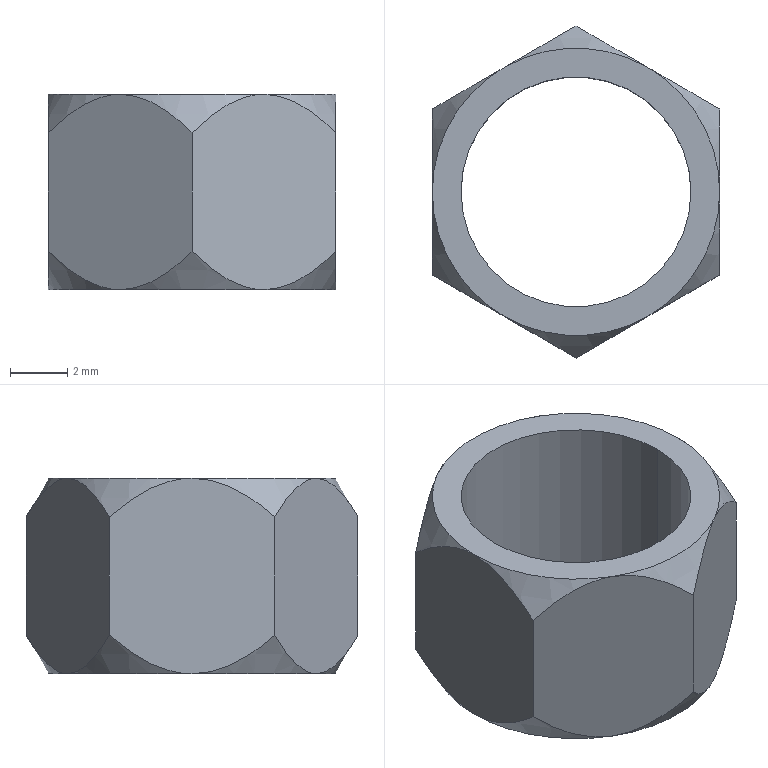Part | SolidWorks | features ICE 2, Extrusion 1, MirrorPattern 1 | 1 solid | 22 faces | box 10 x 11.547 x 6.8 mm | volume 240.578 mm3 | cone 12 | plane 8 | cylinder 2 | commonest cylinder face diameters 8 x2
STEP:
#1=CARTESIAN_POINT('',(-4.,0.,-3.4));
#2=VERTEX_POINT('',#1);
#3=CARTESIAN_POINT('',(4.,0.,-3.4));
#4=VERTEX_POINT('',#3);
#5=CARTESIAN_POINT('',(0.,0.,-3.4));
#6=DIRECTION('',(0.,0.,1.));
#7=DIRECTION('',(1.,0.,0.));
#8=AXIS2_PLACEMENT_3D('',#5,#6,#7);
#9=CIRCLE('',#8,4.);
#10=EDGE_CURVE('',#2,#4,#9,.T.);
#11=ORIENTED_EDGE('',*,*,#10,.F.);
#12=CARTESIAN_POINT('',(-4.,0.,3.4));
#13=VERTEX_POINT('',#12);
#14=CARTESIAN_POINT('',(-4.,0.,-3.4));
#15=DIRECTION('',(0.,0.,1.));
#16=VECTOR('',#15,1000.);
#17=LINE('',#14,#16);
#18=EDGE_CURVE('',#2,#13,#17,.T.);
#19=ORIENTED_EDGE('',*,*,#18,.T.);
#20=CARTESIAN_POINT('',(4.,0.,3.4));
#21=VERTEX_POINT('',#20);
#22=CARTESIAN_POINT('',(0.,0.,3.4));
#23=DIRECTION('',(0.,0.,1.));
#24=DIRECTION('',(1.,0.,0.));
#25=AXIS2_PLACEMENT_3D('',#22,#23,#24);
#26=CIRCLE('',#25,4.);
#27=EDGE_CURVE('',#13,#21,#26,.T.);
#28=ORIENTED_EDGE('',*,*,#27,.T.);
#29=CARTESIAN_POINT('',(4.,0.,-3.4));
#30=DIRECTION('',(0.,0.,1.));
#31=VECTOR('',#30,1000.);
#32=LINE('',#29,#31);
#33=EDGE_CURVE('',#4,#21,#32,.T.);
#34=ORIENTED_EDGE('',*,*,#33,.F.);
#35=EDGE_LOOP('',(#11,#19,#28,#34));
#36=FACE_OUTER_BOUND('',#35,.T.);
#37=CARTESIAN_POINT('',(0.,0.,-3.4));
#38=DIRECTION('',(0.,0.,1.));
#39=DIRECTION('',(1.,0.,0.));
#40=AXIS2_PLACEMENT_3D('',#37,#38,#39);
#41=CYLINDRICAL_SURFACE('',#40,4.);
#42=ADVANCED_FACE('',(#36),#41,.F.);
#43=CARTESIAN_POINT('',(5.,2.887,2.06));
#44=VERTEX_POINT('',#43);
#45=CARTESIAN_POINT('',(5.,2.887,-2.06));
#46=VERTEX_POINT('',#45);
#47=CARTESIAN_POINT('',(5.,2.887,3.4));
#48=DIRECTION('',(0.,0.,-1.));
#49=VECTOR('',#48,1000.);
#50=LINE('',#47,#49);
#51=EDGE_CURVE('',#44,#46,#50,.T.);
#52=ORIENTED_EDGE('',*,*,#51,.T.);
#53=CARTESIAN_POINT('',(2.5,4.33,-3.4));
#54=VERTEX_POINT('',#53);
#55=CARTESIAN_POINT('',(5.,2.887,-2.06));
#56=CARTESIAN_POINT('',(4.644,3.092,-2.416));
#57=CARTESIAN_POINT('',(4.27,3.308,-2.738));
#58=CARTESIAN_POINT('',(3.645,3.669,-3.111));
#59=CARTESIAN_POINT('',(3.424,3.797,-3.216));
#60=CARTESIAN_POINT('',(3.085,3.992,-3.324));
#61=CARTESIAN_POINT('',(2.97,4.059,-3.352));
#62=CARTESIAN_POINT('',(2.737,4.193,-3.39));
#63=CARTESIAN_POINT('',(2.617,4.262,-3.4));
#64=CARTESIAN_POINT('',(2.5,4.33,-3.4));
#65=B_SPLINE_CURVE_WITH_KNOTS('',3,(#55,#56,#57,#58,#59,#60,#61,#62,#63,#64),.UNSPECIFIED.,.F.,.F.,(4,2,2,2,4),(0.000000303,0.001616,0.002424,0.002828,0.003232),.UNSPECIFIED.);
#66=EDGE_CURVE('',#46,#54,#65,.T.);
#67=ORIENTED_EDGE('',*,*,#66,.T.);
#68=CARTESIAN_POINT('',(0.,5.774,-2.06));
#69=VERTEX_POINT('',#68);
#70=CARTESIAN_POINT('',(2.5,4.33,-3.4));
#71=CARTESIAN_POINT('',(2.265,4.466,-3.4));
#72=CARTESIAN_POINT('',(2.034,4.599,-3.362));
#73=CARTESIAN_POINT('',(1.578,4.863,-3.217));
#74=CARTESIAN_POINT('',(1.361,4.988,-3.114));
#75=CARTESIAN_POINT('',(0.9455,5.228,-2.867));
#76=CARTESIAN_POINT('',(0.7456,5.343,-2.723));
#77=CARTESIAN_POINT('',(0.3618,5.565,-2.408));
#78=CARTESIAN_POINT('',(0.1781,5.671,-2.238));
#79=CARTESIAN_POINT('',(0.,5.774,-2.06));
#80=B_SPLINE_CURVE_WITH_KNOTS('',3,(#70,#71,#72,#73,#74,#75,#76,#77,#78,#79),.UNSPECIFIED.,.F.,.F.,(4,2,2,2,4),(0.003232,0.004038,0.004845,0.005652,0.006458),.UNSPECIFIED.);
#81=EDGE_CURVE('',#54,#69,#80,.T.);
#82=ORIENTED_EDGE('',*,*,#81,.T.);
#83=CARTESIAN_POINT('',(0.,5.774,2.06));
#84=VERTEX_POINT('',#83);
#85=CARTESIAN_POINT('',(0.,5.774,3.4));
#86=DIRECTION('',(0.,0.,-1.));
#87=VECTOR('',#86,1000.);
#88=LINE('',#85,#87);
#89=EDGE_CURVE('',#84,#69,#88,.T.);
#90=ORIENTED_EDGE('',*,*,#89,.F.);
#91=CARTESIAN_POINT('',(2.5,4.33,3.4));
#92=VERTEX_POINT('',#91);
#93=CARTESIAN_POINT('',(2.5,4.33,3.4));
#94=CARTESIAN_POINT('',(2.265,4.466,3.4));
#95=CARTESIAN_POINT('',(2.034,4.599,3.362));
#96=CARTESIAN_POINT('',(1.578,4.863,3.217));
#97=CARTESIAN_POINT('',(1.361,4.988,3.114));
#98=CARTESIAN_POINT('',(0.9455,5.228,2.867));
#99=CARTESIAN_POINT('',(0.7456,5.343,2.723));
#100=CARTESIAN_POINT('',(0.3618,5.565,2.408));
#101=CARTESIAN_POINT('',(0.1781,5.671,2.238));
#102=CARTESIAN_POINT('',(0.,5.774,2.06));
#103=B_SPLINE_CURVE_WITH_KNOTS('',3,(#93,#94,#95,#96,#97,#98,#99,#100,#101,#102),.UNSPECIFIED.,.F.,.F.,(4,2,2,2,4),(0.003232,0.004038,0.004845,0.005652,0.006458),.UNSPECIFIED.);
#104=EDGE_CURVE('',#92,#84,#103,.T.);
#105=ORIENTED_EDGE('',*,*,#104,.F.);
#106=CARTESIAN_POINT('',(5.,2.887,2.06));
#107=CARTESIAN_POINT('',(4.644,3.092,2.416));
#108=CARTESIAN_POINT('',(4.27,3.308,2.738));
#109=CARTESIAN_POINT('',(3.645,3.669,3.111));
#110=CARTESIAN_POINT('',(3.424,3.797,3.216));
#111=CARTESIAN_POINT('',(3.085,3.992,3.324));
#112=CARTESIAN_POINT('',(2.97,4.059,3.352));
#113=CARTESIAN_POINT('',(2.737,4.193,3.39));
#114=CARTESIAN_POINT('',(2.617,4.262,3.4));
#115=CARTESIAN_POINT('',(2.5,4.33,3.4));
#116=B_SPLINE_CURVE_WITH_KNOTS('',3,(#106,#107,#108,#109,#110,#111,#112,#113,#114,#115),.UNSPECIFIED.,.F.,.F.,(4,2,2,2,4),(0.000000303,0.001616,0.002424,0.002828,0.003232),.UNSPECIFIED.);
#117=EDGE_CURVE('',#44,#92,#116,.T.);
#118=ORIENTED_EDGE('',*,*,#117,.F.);
#119=EDGE_LOOP('',(#52,#67,#82,#90,#105,#118));
#120=FACE_OUTER_BOUND('',#119,.T.);
#121=CARTESIAN_POINT('',(5.,2.887,3.4));
#122=DIRECTION('',(-0.5,-0.866,0.));
#123=DIRECTION('',(0.866,-0.5,0.));
#124=AXIS2_PLACEMENT_3D('',#121,#122,#123);
#125=PLANE('',#124);
#126=ADVANCED_FACE('',(#120),#125,.F.);
#127=ORIENTED_EDGE('',*,*,#89,.T.);
#128=CARTESIAN_POINT('',(-2.5,4.33,-3.4));
#129=VERTEX_POINT('',#128);
#130=CARTESIAN_POINT('',(0.,5.774,-2.06));
#131=CARTESIAN_POINT('',(-0.3557,5.568,-2.416));
#132=CARTESIAN_POINT('',(-0.7302,5.352,-2.738));
#133=CARTESIAN_POINT('',(-1.355,4.991,-3.111));
#134=CARTESIAN_POINT('',(-1.576,4.864,-3.216));
#135=CARTESIAN_POINT('',(-1.915,4.668,-3.324));
#136=CARTESIAN_POINT('',(-2.03,4.602,-3.352));
#137=CARTESIAN_POINT('',(-2.263,4.467,-3.39));
#138=CARTESIAN_POINT('',(-2.383,4.398,-3.4));
#139=CARTESIAN_POINT('',(-2.5,4.33,-3.4));
#140=B_SPLINE_CURVE_WITH_KNOTS('',3,(#130,#131,#132,#133,#134,#135,#136,#137,#138,#139),.UNSPECIFIED.,.F.,.F.,(4,2,2,2,4),(0.000000303,0.001616,0.002424,0.002828,0.003232),.UNSPECIFIED.);
#141=EDGE_CURVE('',#69,#129,#140,.T.);
#142=ORIENTED_EDGE('',*,*,#141,.T.);
#143=CARTESIAN_POINT('',(-5.,2.887,-2.06));
#144=VERTEX_POINT('',#143);
#145=CARTESIAN_POINT('',(-2.5,4.33,-3.4));
#146=CARTESIAN_POINT('',(-2.735,4.195,-3.4));
#147=CARTESIAN_POINT('',(-2.966,4.061,-3.362));
#148=CARTESIAN_POINT('',(-3.422,3.798,-3.217));
#149=CARTESIAN_POINT('',(-3.639,3.672,-3.114));
#150=CARTESIAN_POINT('',(-4.055,3.433,-2.867));
#151=CARTESIAN_POINT('',(-4.254,3.317,-2.723));
#152=CARTESIAN_POINT('',(-4.638,3.096,-2.408));
#153=CARTESIAN_POINT('',(-4.822,2.99,-2.238));
#154=CARTESIAN_POINT('',(-5.,2.887,-2.06));
#155=B_SPLINE_CURVE_WITH_KNOTS('',3,(#145,#146,#147,#148,#149,#150,#151,#152,#153,#154),.UNSPECIFIED.,.F.,.F.,(4,2,2,2,4),(0.003232,0.004038,0.004845,0.005652,0.006458),.UNSPECIFIED.);
#156=EDGE_CURVE('',#129,#144,#155,.T.);
#157=ORIENTED_EDGE('',*,*,#156,.T.);
#158=CARTESIAN_POINT('',(-5.,2.887,2.06));
#159=VERTEX_POINT('',#158);
#160=CARTESIAN_POINT('',(-5.,2.887,3.4));
#161=DIRECTION('',(0.,0.,-1.));
#162=VECTOR('',#161,1000.);
#163=LINE('',#160,#162);
#164=EDGE_CURVE('',#159,#144,#163,.T.);
#165=ORIENTED_EDGE('',*,*,#164,.F.);
#166=CARTESIAN_POINT('',(-2.5,4.33,3.4));
#167=VERTEX_POINT('',#166);
#168=CARTESIAN_POINT('',(-2.5,4.33,3.4));
#169=CARTESIAN_POINT('',(-2.735,4.195,3.4));
#170=CARTESIAN_POINT('',(-2.966,4.061,3.362));
#171=CARTESIAN_POINT('',(-3.422,3.798,3.217));
#172=CARTESIAN_POINT('',(-3.639,3.672,3.114));
#173=CARTESIAN_POINT('',(-4.055,3.433,2.867));
#174=CARTESIAN_POINT('',(-4.254,3.317,2.723));
#175=CARTESIAN_POINT('',(-4.638,3.096,2.408));
#176=CARTESIAN_POINT('',(-4.822,2.99,2.238));
#177=CARTESIAN_POINT('',(-5.,2.887,2.06));
#178=B_SPLINE_CURVE_WITH_KNOTS('',3,(#168,#169,#170,#171,#172,#173,#174,#175,#176,#177),.UNSPECIFIED.,.F.,.F.,(4,2,2,2,4),(0.003232,0.004038,0.004845,0.005652,0.006458),.UNSPECIFIED.);
#179=EDGE_CURVE('',#167,#159,#178,.T.);
#180=ORIENTED_EDGE('',*,*,#179,.F.);
#181=CARTESIAN_POINT('',(0.,5.774,2.06));
#182=CARTESIAN_POINT('',(-0.3557,5.568,2.416));
#183=CARTESIAN_POINT('',(-0.7302,5.352,2.738));
#184=CARTESIAN_POINT('',(-1.355,4.991,3.111));
#185=CARTESIAN_POINT('',(-1.576,4.864,3.216));
#186=CARTESIAN_POINT('',(-1.915,4.668,3.324));
#187=CARTESIAN_POINT('',(-2.03,4.602,3.352));
#188=CARTESIAN_POINT('',(-2.263,4.467,3.39));
#189=CARTESIAN_POINT('',(-2.383,4.398,3.4));
#190=CARTESIAN_POINT('',(-2.5,4.33,3.4));
#191=B_SPLINE_CURVE_WITH_KNOTS('',3,(#181,#182,#183,#184,#185,#186,#187,#188,#189,#190),.UNSPECIFIED.,.F.,.F.,(4,2,2,2,4),(0.000000303,0.001616,0.002424,0.002828,0.003232),.UNSPECIFIED.);
#192=EDGE_CURVE('',#84,#167,#191,.T.);
#193=ORIENTED_EDGE('',*,*,#192,.F.);
#194=EDGE_LOOP('',(#127,#142,#157,#165,#180,#193));
#195=FACE_OUTER_BOUND('',#194,.T.);
#196=CARTESIAN_POINT('',(0.,5.774,3.4));
#197=DIRECTION('',(0.5,-0.866,0.));
#198=DIRECTION('',(0.866,0.5,0.));
#199=AXIS2_PLACEMENT_3D('',#196,#197,#198);
#200=PLANE('',#199);
#201=ADVANCED_FACE('',(#195),#200,.F.);
#202=ORIENTED_EDGE('',*,*,#164,.T.);
#203=CARTESIAN_POINT('',(-5.,0.,-3.4));
#204=VERTEX_POINT('',#203);
#205=CARTESIAN_POINT('',(-5.,2.887,-2.06));
#206=CARTESIAN_POINT('',(-5.,2.683,-2.237));
#207=CARTESIAN_POINT('',(-5.,2.47,-2.407));
#208=CARTESIAN_POINT('',(-5.,2.029,-2.721));
#209=CARTESIAN_POINT('',(-5.,1.8,-2.864));
#210=CARTESIAN_POINT('',(-5.,1.32,-3.112));
#211=CARTESIAN_POINT('',(-5.,1.066,-3.217));
#212=CARTESIAN_POINT('',(-5.,0.5432,-3.361));
#213=CARTESIAN_POINT('',(-5.,0.2728,-3.4));
#214=CARTESIAN_POINT('',(-5.,0.,-3.4));
#215=B_SPLINE_CURVE_WITH_KNOTS('',3,(#205,#206,#207,#208,#209,#210,#211,#212,#213,#214),.UNSPECIFIED.,.F.,.F.,(4,2,2,2,4),(0.005872,0.006672,0.007473,0.008273,0.009073),.UNSPECIFIED.);
#216=EDGE_CURVE('',#144,#204,#215,.T.);
#217=ORIENTED_EDGE('',*,*,#216,.T.);
#218=CARTESIAN_POINT('',(-5.,-2.887,-2.06));
#219=VERTEX_POINT('',#218);
#220=CARTESIAN_POINT('',(-5.,0.,-3.4));
#221=CARTESIAN_POINT('',(-5.,-0.2731,-3.4));
#222=CARTESIAN_POINT('',(-5.,-0.5406,-3.361));
#223=CARTESIAN_POINT('',(-5.,-1.066,-3.217));
#224=CARTESIAN_POINT('',(-5.,-1.319,-3.113));
#225=CARTESIAN_POINT('',(-5.,-1.799,-2.865));
#226=CARTESIAN_POINT('',(-5.,-2.029,-2.721));
#227=CARTESIAN_POINT('',(-5.,-2.473,-2.405));
#228=CARTESIAN_POINT('',(-5.,-2.683,-2.236));
#229=CARTESIAN_POINT('',(-5.,-2.887,-2.06));
#230=B_SPLINE_CURVE_WITH_KNOTS('',3,(#220,#221,#222,#223,#224,#225,#226,#227,#228,#229),.UNSPECIFIED.,.F.,.F.,(4,2,2,2,4),(0.009073,0.009874,0.01068,0.01148,0.01228),.UNSPECIFIED.);
#231=EDGE_CURVE('',#204,#219,#230,.T.);
#232=ORIENTED_EDGE('',*,*,#231,.T.);
#233=CARTESIAN_POINT('',(-5.,-2.887,2.06));
#234=VERTEX_POINT('',#233);
#235=CARTESIAN_POINT('',(-5.,-2.887,3.4));
#236=DIRECTION('',(0.,0.,-1.));
#237=VECTOR('',#236,1000.);
#238=LINE('',#235,#237);
#239=EDGE_CURVE('',#234,#219,#238,.T.);
#240=ORIENTED_EDGE('',*,*,#239,.F.);
#241=CARTESIAN_POINT('',(-5.,0.,3.4));
#242=VERTEX_POINT('',#241);
#243=CARTESIAN_POINT('',(-5.,0.,3.4));
#244=CARTESIAN_POINT('',(-5.,-0.273,3.4));
#245=CARTESIAN_POINT('',(-5.,-0.5406,3.361));
#246=CARTESIAN_POINT('',(-5.,-1.066,3.217));
#247=CARTESIAN_POINT('',(-5.,-1.319,3.113));
#248=CARTESIAN_POINT('',(-5.,-1.799,2.865));
#249=CARTESIAN_POINT('',(-5.,-2.029,2.72));
#250=CARTESIAN_POINT('',(-5.,-2.473,2.405));
#251=CARTESIAN_POINT('',(-5.,-2.683,2.236));
#252=CARTESIAN_POINT('',(-5.,-2.887,2.06));
#253=B_SPLINE_CURVE_WITH_KNOTS('',3,(#243,#244,#245,#246,#247,#248,#249,#250,#251,#252),.UNSPECIFIED.,.F.,.F.,(4,2,2,2,4),(0.009122,0.009923,0.01072,0.01153,0.01233),.UNSPECIFIED.);
#254=EDGE_CURVE('',#242,#234,#253,.T.);
#255=ORIENTED_EDGE('',*,*,#254,.F.);
#256=CARTESIAN_POINT('',(-5.,2.887,2.06));
#257=CARTESIAN_POINT('',(-5.,2.683,2.237));
#258=CARTESIAN_POINT('',(-5.,2.47,2.407));
#259=CARTESIAN_POINT('',(-5.,2.029,2.721));
#260=CARTESIAN_POINT('',(-5.,1.8,2.864));
#261=CARTESIAN_POINT('',(-5.,1.32,3.112));
#262=CARTESIAN_POINT('',(-5.,1.066,3.217));
#263=CARTESIAN_POINT('',(-5.,0.5432,3.361));
#264=CARTESIAN_POINT('',(-5.,0.2728,3.4));
#265=CARTESIAN_POINT('',(-5.,0.,3.4));
#266=B_SPLINE_CURVE_WITH_KNOTS('',3,(#256,#257,#258,#259,#260,#261,#262,#263,#264,#265),.UNSPECIFIED.,.F.,.F.,(4,2,2,2,4),(0.005921,0.006721,0.007521,0.008322,0.009122),.UNSPECIFIED.);
#267=EDGE_CURVE('',#159,#242,#266,.T.);
#268=ORIENTED_EDGE('',*,*,#267,.F.);
#269=EDGE_LOOP('',(#202,#217,#232,#240,#255,#268));
#270=FACE_OUTER_BOUND('',#269,.T.);
#271=CARTESIAN_POINT('',(-5.,2.887,3.4));
#272=DIRECTION('',(1.,0.,0.));
#273=DIRECTION('',(0.,1.,0.));
#274=AXIS2_PLACEMENT_3D('',#271,#272,#273);
#275=PLANE('',#274);
#276=ADVANCED_FACE('',(#270),#275,.F.);
#277=ORIENTED_EDGE('',*,*,#239,.T.);
#278=CARTESIAN_POINT('',(-2.5,-4.33,-3.4));
#279=VERTEX_POINT('',#278);
#280=CARTESIAN_POINT('',(-5.,-2.887,-2.06));
#281=CARTESIAN_POINT('',(-4.644,-3.092,-2.416));
#282=CARTESIAN_POINT('',(-4.27,-3.308,-2.738));
#283=CARTESIAN_POINT('',(-3.645,-3.669,-3.111));
#284=CARTESIAN_POINT('',(-3.424,-3.797,-3.216));
#285=CARTESIAN_POINT('',(-3.085,-3.992,-3.324));
#286=CARTESIAN_POINT('',(-2.97,-4.059,-3.352));
#287=CARTESIAN_POINT('',(-2.737,-4.193,-3.39));
#288=CARTESIAN_POINT('',(-2.617,-4.262,-3.4));
#289=CARTESIAN_POINT('',(-2.5,-4.33,-3.4));
#290=B_SPLINE_CURVE_WITH_KNOTS('',3,(#280,#281,#282,#283,#284,#285,#286,#287,#288,#289),.UNSPECIFIED.,.F.,.F.,(4,2,2,2,4),(0.000000303,0.001616,0.002424,0.002828,0.003232),.UNSPECIFIED.);
#291=EDGE_CURVE('',#219,#279,#290,.T.);
#292=ORIENTED_EDGE('',*,*,#291,.T.);
#293=CARTESIAN_POINT('',(0.,-5.774,-2.06));
#294=VERTEX_POINT('',#293);
#295=CARTESIAN_POINT('',(-2.5,-4.33,-3.4));
#296=CARTESIAN_POINT('',(-2.265,-4.466,-3.4));
#297=CARTESIAN_POINT('',(-2.034,-4.599,-3.362));
#298=CARTESIAN_POINT('',(-1.578,-4.863,-3.217));
#299=CARTESIAN_POINT('',(-1.361,-4.988,-3.114));
#300=CARTESIAN_POINT('',(-0.9455,-5.228,-2.867));
#301=CARTESIAN_POINT('',(-0.7456,-5.343,-2.723));
#302=CARTESIAN_POINT('',(-0.3618,-5.565,-2.408));
#303=CARTESIAN_POINT('',(-0.1781,-5.671,-2.238));
#304=CARTESIAN_POINT('',(0.,-5.774,-2.06));
#305=B_SPLINE_CURVE_WITH_KNOTS('',3,(#295,#296,#297,#298,#299,#300,#301,#302,#303,#304),.UNSPECIFIED.,.F.,.F.,(4,2,2,2,4),(0.003232,0.004038,0.004845,0.005652,0.006458),.UNSPECIFIED.);
#306=EDGE_CURVE('',#279,#294,#305,.T.);
#307=ORIENTED_EDGE('',*,*,#306,.T.);
#308=CARTESIAN_POINT('',(0.,-5.774,2.06));
#309=VERTEX_POINT('',#308);
#310=CARTESIAN_POINT('',(0.,-5.774,3.4));
#311=DIRECTION('',(0.,0.,-1.));
#312=VECTOR('',#311,1000.);
#313=LINE('',#310,#312);
#314=EDGE_CURVE('',#309,#294,#313,.T.);
#315=ORIENTED_EDGE('',*,*,#314,.F.);
#316=CARTESIAN_POINT('',(-2.5,-4.33,3.4));
#317=VERTEX_POINT('',#316);
#318=CARTESIAN_POINT('',(-2.5,-4.33,3.4));
#319=CARTESIAN_POINT('',(-2.265,-4.466,3.4));
#320=CARTESIAN_POINT('',(-2.034,-4.599,3.362));
#321=CARTESIAN_POINT('',(-1.578,-4.863,3.217));
#322=CARTESIAN_POINT('',(-1.361,-4.988,3.114));
#323=CARTESIAN_POINT('',(-0.9455,-5.228,2.867));
#324=CARTESIAN_POINT('',(-0.7456,-5.343,2.723));
#325=CARTESIAN_POINT('',(-0.3618,-5.565,2.408));
#326=CARTESIAN_POINT('',(-0.1781,-5.671,2.238));
#327=CARTESIAN_POINT('',(0.,-5.774,2.06));
#328=B_SPLINE_CURVE_WITH_KNOTS('',3,(#318,#319,#320,#321,#322,#323,#324,#325,#326,#327),.UNSPECIFIED.,.F.,.F.,(4,2,2,2,4),(0.003232,0.004038,0.004845,0.005652,0.006458),.UNSPECIFIED.);
#329=EDGE_CURVE('',#317,#309,#328,.T.);
#330=ORIENTED_EDGE('',*,*,#329,.F.);
#331=CARTESIAN_POINT('',(-5.,-2.887,2.06));
#332=CARTESIAN_POINT('',(-4.644,-3.092,2.416));
#333=CARTESIAN_POINT('',(-4.27,-3.308,2.738));
#334=CARTESIAN_POINT('',(-3.645,-3.669,3.111));
#335=CARTESIAN_POINT('',(-3.424,-3.797,3.216));
#336=CARTESIAN_POINT('',(-3.085,-3.992,3.324));
#337=CARTESIAN_POINT('',(-2.97,-4.059,3.352));
#338=CARTESIAN_POINT('',(-2.737,-4.193,3.39));
#339=CARTESIAN_POINT('',(-2.617,-4.262,3.4));
#340=CARTESIAN_POINT('',(-2.5,-4.33,3.4));
#341=B_SPLINE_CURVE_WITH_KNOTS('',3,(#331,#332,#333,#334,#335,#336,#337,#338,#339,#340),.UNSPECIFIED.,.F.,.F.,(4,2,2,2,4),(0.000000303,0.001616,0.002424,0.002828,0.003232),.UNSPECIFIED.);
#342=EDGE_CURVE('',#234,#317,#341,.T.);
#343=ORIENTED_EDGE('',*,*,#342,.F.);
#344=EDGE_LOOP('',(#277,#292,#307,#315,#330,#343));
#345=FACE_OUTER_BOUND('',#344,.T.);
#346=CARTESIAN_POINT('',(-5.,-2.887,3.4));
#347=DIRECTION('',(0.5,0.866,0.));
#348=DIRECTION('',(-0.866,0.5,0.));
#349=AXIS2_PLACEMENT_3D('',#346,#347,#348);
#350=PLANE('',#349);
#351=ADVANCED_FACE('',(#345),#350,.F.);
#352=ORIENTED_EDGE('',*,*,#314,.T.);
#353=CARTESIAN_POINT('',(2.5,-4.33,-3.4));
#354=VERTEX_POINT('',#353);
#355=CARTESIAN_POINT('',(0.,-5.774,-2.06));
#356=CARTESIAN_POINT('',(0.3557,-5.568,-2.416));
#357=CARTESIAN_POINT('',(0.7302,-5.352,-2.738));
#358=CARTESIAN_POINT('',(1.355,-4.991,-3.111));
#359=CARTESIAN_POINT('',(1.576,-4.864,-3.216));
#360=CARTESIAN_POINT('',(1.915,-4.668,-3.324));
#361=CARTESIAN_POINT('',(2.03,-4.602,-3.352));
#362=CARTESIAN_POINT('',(2.263,-4.467,-3.39));
#363=CARTESIAN_POINT('',(2.383,-4.398,-3.4));
#364=CARTESIAN_POINT('',(2.5,-4.33,-3.4));
#365=B_SPLINE_CURVE_WITH_KNOTS('',3,(#355,#356,#357,#358,#359,#360,#361,#362,#363,#364),.UNSPECIFIED.,.F.,.F.,(4,2,2,2,4),(0.000000303,0.001616,0.002424,0.002828,0.003232),.UNSPECIFIED.);
#366=EDGE_CURVE('',#294,#354,#365,.T.);
#367=ORIENTED_EDGE('',*,*,#366,.T.);
#368=CARTESIAN_POINT('',(5.,-2.887,-2.06));
#369=VERTEX_POINT('',#368);
#370=CARTESIAN_POINT('',(2.5,-4.33,-3.4));
#371=CARTESIAN_POINT('',(2.735,-4.195,-3.4));
#372=CARTESIAN_POINT('',(2.966,-4.061,-3.362));
#373=CARTESIAN_POINT('',(3.422,-3.798,-3.217));
#374=CARTESIAN_POINT('',(3.639,-3.672,-3.114));
#375=CARTESIAN_POINT('',(4.055,-3.433,-2.867));
#376=CARTESIAN_POINT('',(4.254,-3.317,-2.723));
#377=CARTESIAN_POINT('',(4.638,-3.096,-2.408));
#378=CARTESIAN_POINT('',(4.822,-2.99,-2.238));
#379=CARTESIAN_POINT('',(5.,-2.887,-2.06));
#380=B_SPLINE_CURVE_WITH_KNOTS('',3,(#370,#371,#372,#373,#374,#375,#376,#377,#378,#379),.UNSPECIFIED.,.F.,.F.,(4,2,2,2,4),(0.003232,0.004038,0.004845,0.005652,0.006458),.UNSPECIFIED.);
#381=EDGE_CURVE('',#354,#369,#380,.T.);
#382=ORIENTED_EDGE('',*,*,#381,.T.);
#383=CARTESIAN_POINT('',(5.,-2.887,2.06));
#384=VERTEX_POINT('',#383);
#385=CARTESIAN_POINT('',(5.,-2.887,3.4));
#386=DIRECTION('',(0.,0.,-1.));
#387=VECTOR('',#386,1000.);
#388=LINE('',#385,#387);
#389=EDGE_CURVE('',#384,#369,#388,.T.);
#390=ORIENTED_EDGE('',*,*,#389,.F.);
#391=CARTESIAN_POINT('',(2.5,-4.33,3.4));
#392=VERTEX_POINT('',#391);
#393=CARTESIAN_POINT('',(2.5,-4.33,3.4));
#394=CARTESIAN_POINT('',(2.735,-4.195,3.4));
#395=CARTESIAN_POINT('',(2.966,-4.061,3.362));
#396=CARTESIAN_POINT('',(3.422,-3.798,3.217));
#397=CARTESIAN_POINT('',(3.639,-3.672,3.114));
#398=CARTESIAN_POINT('',(4.055,-3.433,2.867));
#399=CARTESIAN_POINT('',(4.254,-3.317,2.723));
#400=CARTESIAN_POINT('',(4.638,-3.096,2.408));
#401=CARTESIAN_POINT('',(4.822,-2.99,2.238));
#402=CARTESIAN_POINT('',(5.,-2.887,2.06));
#403=B_SPLINE_CURVE_WITH_KNOTS('',3,(#393,#394,#395,#396,#397,#398,#399,#400,#401,#402),.UNSPECIFIED.,.F.,.F.,(4,2,2,2,4),(0.003232,0.004038,0.004845,0.005652,0.006458),.UNSPECIFIED.);
#404=EDGE_CURVE('',#392,#384,#403,.T.);
#405=ORIENTED_EDGE('',*,*,#404,.F.);
#406=CARTESIAN_POINT('',(0.,-5.774,2.06));
#407=CARTESIAN_POINT('',(0.3557,-5.568,2.416));
#408=CARTESIAN_POINT('',(0.7302,-5.352,2.738));
#409=CARTESIAN_POINT('',(1.355,-4.991,3.111));
#410=CARTESIAN_POINT('',(1.576,-4.864,3.216));
#411=CARTESIAN_POINT('',(1.915,-4.668,3.324));
#412=CARTESIAN_POINT('',(2.03,-4.602,3.352));
#413=CARTESIAN_POINT('',(2.263,-4.467,3.39));
#414=CARTESIAN_POINT('',(2.383,-4.398,3.4));
#415=CARTESIAN_POINT('',(2.5,-4.33,3.4));
#416=B_SPLINE_CURVE_WITH_KNOTS('',3,(#406,#407,#408,#409,#410,#411,#412,#413,#414,#415),.UNSPECIFIED.,.F.,.F.,(4,2,2,2,4),(0.000000303,0.001616,0.002424,0.002828,0.003232),.UNSPECIFIED.);
#417=EDGE_CURVE('',#309,#392,#416,.T.);
#418=ORIENTED_EDGE('',*,*,#417,.F.);
#419=EDGE_LOOP('',(#352,#367,#382,#390,#405,#418));
#420=FACE_OUTER_BOUND('',#419,.T.);
#421=CARTESIAN_POINT('',(0.,-5.774,3.4));
#422=DIRECTION('',(-0.5,0.866,0.));
#423=DIRECTION('',(-0.866,-0.5,0.));
#424=AXIS2_PLACEMENT_3D('',#421,#422,#423);
#425=PLANE('',#424);
#426=ADVANCED_FACE('',(#420),#425,.F.);
#427=ORIENTED_EDGE('',*,*,#389,.T.);
#428=CARTESIAN_POINT('',(5.,0.,-3.4));
#429=VERTEX_POINT('',#428);
#430=CARTESIAN_POINT('',(5.,-2.887,-2.06));
#431=CARTESIAN_POINT('',(5.,-2.683,-2.236));
#432=CARTESIAN_POINT('',(5.,-2.473,-2.405));
#433=CARTESIAN_POINT('',(5.,-2.029,-2.721));
#434=CARTESIAN_POINT('',(5.,-1.799,-2.865));
#435=CARTESIAN_POINT('',(5.,-1.319,-3.113));
#436=CARTESIAN_POINT('',(5.,-1.066,-3.217));
#437=CARTESIAN_POINT('',(5.,-0.5406,-3.361));
#438=CARTESIAN_POINT('',(5.,-0.2731,-3.4));
#439=CARTESIAN_POINT('',(5.,0.,-3.4));
#440=B_SPLINE_CURVE_WITH_KNOTS('',3,(#430,#431,#432,#433,#434,#435,#436,#437,#438,#439),.UNSPECIFIED.,.F.,.F.,(4,2,2,2,4),(0.02011,0.02091,0.02172,0.02253,0.02333),.UNSPECIFIED.);
#441=EDGE_CURVE('',#369,#429,#440,.T.);
#442=ORIENTED_EDGE('',*,*,#441,.T.);
#443=CARTESIAN_POINT('',(5.,0.,-3.4));
#444=CARTESIAN_POINT('',(5.,0.2728,-3.4));
#445=CARTESIAN_POINT('',(5.,0.5432,-3.361));
#446=CARTESIAN_POINT('',(5.,1.066,-3.217));
#447=CARTESIAN_POINT('',(5.,1.32,-3.112));
#448=CARTESIAN_POINT('',(5.,1.8,-2.864));
#449=CARTESIAN_POINT('',(5.,2.029,-2.721));
#450=CARTESIAN_POINT('',(5.,2.47,-2.407));
#451=CARTESIAN_POINT('',(5.,2.683,-2.237));
#452=CARTESIAN_POINT('',(5.,2.887,-2.06));
#453=B_SPLINE_CURVE_WITH_KNOTS('',3,(#443,#444,#445,#446,#447,#448,#449,#450,#451,#452),.UNSPECIFIED.,.F.,.F.,(4,2,2,2,4),(0.02333,0.02414,0.02494,0.02575,0.02655),.UNSPECIFIED.);
#454=EDGE_CURVE('',#429,#46,#453,.T.);
#455=ORIENTED_EDGE('',*,*,#454,.T.);
#456=ORIENTED_EDGE('',*,*,#51,.F.);
#457=CARTESIAN_POINT('',(5.,0.,3.4));
#458=VERTEX_POINT('',#457);
#459=CARTESIAN_POINT('',(5.,0.,3.4));
#460=CARTESIAN_POINT('',(5.,0.2728,3.4));
#461=CARTESIAN_POINT('',(5.,0.5432,3.361));
#462=CARTESIAN_POINT('',(5.,1.066,3.217));
#463=CARTESIAN_POINT('',(5.,1.32,3.112));
#464=CARTESIAN_POINT('',(5.,1.8,2.864));
#465=CARTESIAN_POINT('',(5.,2.029,2.721));
#466=CARTESIAN_POINT('',(5.,2.47,2.407));
#467=CARTESIAN_POINT('',(5.,2.683,2.237));
#468=CARTESIAN_POINT('',(5.,2.887,2.06));
#469=B_SPLINE_CURVE_WITH_KNOTS('',3,(#459,#460,#461,#462,#463,#464,#465,#466,#467,#468),.UNSPECIFIED.,.F.,.F.,(4,2,2,2,4),(0.02293,0.02373,0.02454,0.02534,0.02615),.UNSPECIFIED.);
#470=EDGE_CURVE('',#458,#44,#469,.T.);
#471=ORIENTED_EDGE('',*,*,#470,.F.);
#472=CARTESIAN_POINT('',(5.,-2.887,2.06));
#473=CARTESIAN_POINT('',(5.,-2.683,2.236));
#474=CARTESIAN_POINT('',(5.,-2.473,2.405));
#475=CARTESIAN_POINT('',(5.,-2.029,2.72));
#476=CARTESIAN_POINT('',(5.,-1.799,2.865));
#477=CARTESIAN_POINT('',(5.,-1.319,3.113));
#478=CARTESIAN_POINT('',(5.,-1.066,3.217));
#479=CARTESIAN_POINT('',(5.,-0.5406,3.361));
#480=CARTESIAN_POINT('',(5.,-0.273,3.4));
#481=CARTESIAN_POINT('',(5.,0.,3.4));
#482=B_SPLINE_CURVE_WITH_KNOTS('',3,(#472,#473,#474,#475,#476,#477,#478,#479,#480,#481),.UNSPECIFIED.,.F.,.F.,(4,2,2,2,4),(0.0197,0.02051,0.02131,0.02212,0.02293),.UNSPECIFIED.);
#483=EDGE_CURVE('',#384,#458,#482,.T.);
#484=ORIENTED_EDGE('',*,*,#483,.F.);
#485=EDGE_LOOP('',(#427,#442,#455,#456,#471,#484));
#486=FACE_OUTER_BOUND('',#485,.T.);
#487=CARTESIAN_POINT('',(5.,-2.887,3.4));
#488=DIRECTION('',(-1.,0.,0.));
#489=DIRECTION('',(0.,-1.,0.));
#490=AXIS2_PLACEMENT_3D('',#487,#488,#489);
#491=PLANE('',#490);
#492=ADVANCED_FACE('',(#486),#491,.F.);
#493=ORIENTED_EDGE('',*,*,#404,.T.);
#494=ORIENTED_EDGE('',*,*,#483,.T.);
#495=CARTESIAN_POINT('',(0.,0.,3.4));
#496=DIRECTION('',(0.,0.,1.));
#497=DIRECTION('',(1.,0.,0.));
#498=AXIS2_PLACEMENT_3D('',#495,#496,#497);
#499=CIRCLE('',#498,5.);
#500=EDGE_CURVE('',#392,#458,#499,.T.);
#501=ORIENTED_EDGE('',*,*,#500,.F.);
#502=EDGE_LOOP('',(#493,#494,#501));
#503=FACE_OUTER_BOUND('',#502,.T.);
#504=CARTESIAN_POINT('',(0.,0.,3.4));
#505=DIRECTION('',(0.,0.,-1.));
#506=DIRECTION('',(1.,0.,0.));
#507=AXIS2_PLACEMENT_3D('',#504,#505,#506);
#508=CONICAL_SURFACE('',#507,5.,0.5236);
#509=ADVANCED_FACE('',(#503),#508,.T.);
#510=ORIENTED_EDGE('',*,*,#329,.T.);
#511=ORIENTED_EDGE('',*,*,#417,.T.);
#512=CARTESIAN_POINT('',(0.,0.,3.4));
#513=DIRECTION('',(0.,0.,1.));
#514=DIRECTION('',(1.,0.,0.));
#515=AXIS2_PLACEMENT_3D('',#512,#513,#514);
#516=CIRCLE('',#515,5.);
#517=EDGE_CURVE('',#317,#392,#516,.T.);
#518=ORIENTED_EDGE('',*,*,#517,.F.);
#519=EDGE_LOOP('',(#510,#511,#518));
#520=FACE_OUTER_BOUND('',#519,.T.);
#521=CARTESIAN_POINT('',(0.,0.,3.4));
#522=DIRECTION('',(0.,0.,-1.));
#523=DIRECTION('',(1.,0.,0.));
#524=AXIS2_PLACEMENT_3D('',#521,#522,#523);
#525=CONICAL_SURFACE('',#524,5.,0.5236);
#526=ADVANCED_FACE('',(#520),#525,.T.);
#527=ORIENTED_EDGE('',*,*,#254,.T.);
#528=ORIENTED_EDGE('',*,*,#342,.T.);
#529=CARTESIAN_POINT('',(0.,0.,3.4));
#530=DIRECTION('',(0.,0.,1.));
#531=DIRECTION('',(1.,0.,0.));
#532=AXIS2_PLACEMENT_3D('',#529,#530,#531);
#533=CIRCLE('',#532,5.);
#534=EDGE_CURVE('',#242,#317,#533,.T.);
#535=ORIENTED_EDGE('',*,*,#534,.F.);
#536=EDGE_LOOP('',(#527,#528,#535));
#537=FACE_OUTER_BOUND('',#536,.T.);
#538=CARTESIAN_POINT('',(0.,0.,3.4));
#539=DIRECTION('',(0.,0.,-1.));
#540=DIRECTION('',(1.,0.,0.));
#541=AXIS2_PLACEMENT_3D('',#538,#539,#540);
#542=CONICAL_SURFACE('',#541,5.,0.5236);
#543=ADVANCED_FACE('',(#537),#542,.T.);
#544=ORIENTED_EDGE('',*,*,#179,.T.);
#545=ORIENTED_EDGE('',*,*,#267,.T.);
#546=CARTESIAN_POINT('',(0.,0.,3.4));
#547=DIRECTION('',(0.,0.,1.));
#548=DIRECTION('',(1.,0.,0.));
#549=AXIS2_PLACEMENT_3D('',#546,#547,#548);
#550=CIRCLE('',#549,5.);
#551=EDGE_CURVE('',#167,#242,#550,.T.);
#552=ORIENTED_EDGE('',*,*,#551,.F.);
#553=EDGE_LOOP('',(#544,#545,#552));
#554=FACE_OUTER_BOUND('',#553,.T.);
#555=CARTESIAN_POINT('',(0.,0.,3.4));
#556=DIRECTION('',(0.,0.,-1.));
#557=DIRECTION('',(1.,0.,0.));
#558=AXIS2_PLACEMENT_3D('',#555,#556,#557);
#559=CONICAL_SURFACE('',#558,5.,0.5236);
#560=ADVANCED_FACE('',(#554),#559,.T.);
#561=ORIENTED_EDGE('',*,*,#104,.T.);
#562=ORIENTED_EDGE('',*,*,#192,.T.);
#563=CARTESIAN_POINT('',(0.,0.,3.4));
#564=DIRECTION('',(0.,0.,1.));
#565=DIRECTION('',(1.,0.,0.));
#566=AXIS2_PLACEMENT_3D('',#563,#564,#565);
#567=CIRCLE('',#566,5.);
#568=EDGE_CURVE('',#92,#167,#567,.T.);
#569=ORIENTED_EDGE('',*,*,#568,.F.);
#570=EDGE_LOOP('',(#561,#562,#569));
#571=FACE_OUTER_BOUND('',#570,.T.);
#572=CARTESIAN_POINT('',(0.,0.,3.4));
#573=DIRECTION('',(0.,0.,-1.));
#574=DIRECTION('',(1.,0.,0.));
#575=AXIS2_PLACEMENT_3D('',#572,#573,#574);
#576=CONICAL_SURFACE('',#575,5.,0.5236);
#577=ADVANCED_FACE('',(#571),#576,.T.);
#578=ORIENTED_EDGE('',*,*,#117,.T.);
#579=CARTESIAN_POINT('',(0.,0.,3.4));
#580=DIRECTION('',(0.,0.,1.));
#581=DIRECTION('',(1.,0.,0.));
#582=AXIS2_PLACEMENT_3D('',#579,#580,#581);
#583=CIRCLE('',#582,5.);
#584=EDGE_CURVE('',#458,#92,#583,.T.);
#585=ORIENTED_EDGE('',*,*,#584,.F.);
#586=ORIENTED_EDGE('',*,*,#470,.T.);
#587=EDGE_LOOP('',(#578,#585,#586));
#588=FACE_OUTER_BOUND('',#587,.T.);
#589=CARTESIAN_POINT('',(0.,0.,3.4));
#590=DIRECTION('',(0.,0.,-1.));
#591=DIRECTION('',(1.,0.,0.));
#592=AXIS2_PLACEMENT_3D('',#589,#590,#591);
#593=CONICAL_SURFACE('',#592,5.,0.5236);
#594=ADVANCED_FACE('',(#588),#593,.T.);
#595=CARTESIAN_POINT('',(0.,0.,3.4));
#596=DIRECTION('',(0.,0.,1.));
#597=DIRECTION('',(1.,0.,0.));
#598=AXIS2_PLACEMENT_3D('',#595,#596,#597);
#599=CIRCLE('',#598,4.);
#600=EDGE_CURVE('',#21,#13,#599,.T.);
#601=ORIENTED_EDGE('',*,*,#600,.F.);
#602=ORIENTED_EDGE('',*,*,#27,.F.);
#603=EDGE_LOOP('',(#601,#602));
#604=FACE_BOUND('',#603,.T.);
#605=ORIENTED_EDGE('',*,*,#500,.T.);
#606=ORIENTED_EDGE('',*,*,#584,.T.);
#607=ORIENTED_EDGE('',*,*,#568,.T.);
#608=ORIENTED_EDGE('',*,*,#551,.T.);
#609=ORIENTED_EDGE('',*,*,#534,.T.);
#610=ORIENTED_EDGE('',*,*,#517,.T.);
#611=EDGE_LOOP('',(#605,#606,#607,#608,#609,#610));
#612=FACE_OUTER_BOUND('',#611,.T.);
#613=CARTESIAN_POINT('',(0.,0.,3.4));
#614=DIRECTION('',(0.,0.,1.));
#615=DIRECTION('',(1.,0.,0.));
#616=AXIS2_PLACEMENT_3D('',#613,#614,#615);
#617=PLANE('',#616);
#618=ADVANCED_FACE('',(#604,#612),#617,.T.);
#619=ORIENTED_EDGE('',*,*,#454,.F.);
#620=CARTESIAN_POINT('',(0.,0.,-3.4));
#621=DIRECTION('',(0.,0.,1.));
#622=DIRECTION('',(1.,0.,0.));
#623=AXIS2_PLACEMENT_3D('',#620,#621,#622);
#624=CIRCLE('',#623,5.);
#625=EDGE_CURVE('',#429,#54,#624,.T.);
#626=ORIENTED_EDGE('',*,*,#625,.T.);
#627=ORIENTED_EDGE('',*,*,#66,.F.);
#628=EDGE_LOOP('',(#619,#626,#627));
#629=FACE_OUTER_BOUND('',#628,.T.);
#630=CARTESIAN_POINT('',(0.,0.,-3.4));
#631=DIRECTION('',(0.,0.,1.));
#632=DIRECTION('',(1.,0.,0.));
#633=AXIS2_PLACEMENT_3D('',#630,#631,#632);
#634=CONICAL_SURFACE('',#633,5.,0.5236);
#635=ADVANCED_FACE('',(#629),#634,.T.);
#636=CARTESIAN_POINT('',(0.,0.,-3.4));
#637=DIRECTION('',(0.,0.,-1.));
#638=DIRECTION('',(1.,0.,0.));
#639=AXIS2_PLACEMENT_3D('',#636,#637,#638);
#640=CIRCLE('',#639,5.);
#641=EDGE_CURVE('',#129,#54,#640,.T.);
#642=ORIENTED_EDGE('',*,*,#641,.F.);
#643=ORIENTED_EDGE('',*,*,#141,.F.);
#644=ORIENTED_EDGE('',*,*,#81,.F.);
#645=EDGE_LOOP('',(#642,#643,#644));
#646=FACE_OUTER_BOUND('',#645,.T.);
#647=CARTESIAN_POINT('',(0.,0.,-3.4));
#648=DIRECTION('',(0.,0.,1.));
#649=DIRECTION('',(1.,0.,0.));
#650=AXIS2_PLACEMENT_3D('',#647,#648,#649);
#651=CONICAL_SURFACE('',#650,5.,0.5236);
#652=ADVANCED_FACE('',(#646),#651,.T.);
#653=CARTESIAN_POINT('',(0.,0.,-3.4));
#654=DIRECTION('',(0.,0.,-1.));
#655=DIRECTION('',(1.,0.,0.));
#656=AXIS2_PLACEMENT_3D('',#653,#654,#655);
#657=CIRCLE('',#656,5.);
#658=EDGE_CURVE('',#204,#129,#657,.T.);
#659=ORIENTED_EDGE('',*,*,#658,.F.);
#660=ORIENTED_EDGE('',*,*,#216,.F.);
#661=ORIENTED_EDGE('',*,*,#156,.F.);
#662=EDGE_LOOP('',(#659,#660,#661));
#663=FACE_OUTER_BOUND('',#662,.T.);
#664=CARTESIAN_POINT('',(0.,0.,-3.4));
#665=DIRECTION('',(0.,0.,1.));
#666=DIRECTION('',(1.,0.,0.));
#667=AXIS2_PLACEMENT_3D('',#664,#665,#666);
#668=CONICAL_SURFACE('',#667,5.,0.5236);
#669=ADVANCED_FACE('',(#663),#668,.T.);
#670=CARTESIAN_POINT('',(0.,0.,-3.4));
#671=DIRECTION('',(0.,0.,-1.));
#672=DIRECTION('',(1.,0.,0.));
#673=AXIS2_PLACEMENT_3D('',#670,#671,#672);
#674=CIRCLE('',#673,5.);
#675=EDGE_CURVE('',#279,#204,#674,.T.);
#676=ORIENTED_EDGE('',*,*,#675,.F.);
#677=ORIENTED_EDGE('',*,*,#291,.F.);
#678=ORIENTED_EDGE('',*,*,#231,.F.);
#679=EDGE_LOOP('',(#676,#677,#678));
#680=FACE_OUTER_BOUND('',#679,.T.);
#681=CARTESIAN_POINT('',(0.,0.,-3.4));
#682=DIRECTION('',(0.,0.,1.));
#683=DIRECTION('',(1.,0.,0.));
#684=AXIS2_PLACEMENT_3D('',#681,#682,#683);
#685=CONICAL_SURFACE('',#684,5.,0.5236);
#686=ADVANCED_FACE('',(#680),#685,.T.);
#687=CARTESIAN_POINT('',(0.,0.,-3.4));
#688=DIRECTION('',(0.,0.,-1.));
#689=DIRECTION('',(1.,0.,0.));
#690=AXIS2_PLACEMENT_3D('',#687,#688,#689);
#691=CIRCLE('',#690,5.);
#692=EDGE_CURVE('',#354,#279,#691,.T.);
#693=ORIENTED_EDGE('',*,*,#692,.F.);
#694=ORIENTED_EDGE('',*,*,#366,.F.);
#695=ORIENTED_EDGE('',*,*,#306,.F.);
#696=EDGE_LOOP('',(#693,#694,#695));
#697=FACE_OUTER_BOUND('',#696,.T.);
#698=CARTESIAN_POINT('',(0.,0.,-3.4));
#699=DIRECTION('',(0.,0.,1.));
#700=DIRECTION('',(1.,0.,0.));
#701=AXIS2_PLACEMENT_3D('',#698,#699,#700);
#702=CONICAL_SURFACE('',#701,5.,0.5236);
#703=ADVANCED_FACE('',(#697),#702,.T.);
#704=CARTESIAN_POINT('',(0.,0.,-3.4));
#705=DIRECTION('',(0.,0.,-1.));
#706=DIRECTION('',(1.,0.,0.));
#707=AXIS2_PLACEMENT_3D('',#704,#705,#706);
#708=CIRCLE('',#707,5.);
#709=EDGE_CURVE('',#429,#354,#708,.T.);
#710=ORIENTED_EDGE('',*,*,#709,.F.);
#711=ORIENTED_EDGE('',*,*,#441,.F.);
#712=ORIENTED_EDGE('',*,*,#381,.F.);
#713=EDGE_LOOP('',(#710,#711,#712));
#714=FACE_OUTER_BOUND('',#713,.T.);
#715=CARTESIAN_POINT('',(0.,0.,-3.4));
#716=DIRECTION('',(0.,0.,1.));
#717=DIRECTION('',(1.,0.,0.));
#718=AXIS2_PLACEMENT_3D('',#715,#716,#717);
#719=CONICAL_SURFACE('',#718,5.,0.5236);
#720=ADVANCED_FACE('',(#714),#719,.T.);
#721=CARTESIAN_POINT('',(0.,0.,-3.4));
#722=DIRECTION('',(0.,0.,1.));
#723=DIRECTION('',(1.,0.,0.));
#724=AXIS2_PLACEMENT_3D('',#721,#722,#723);
#725=CIRCLE('',#724,4.);
#726=EDGE_CURVE('',#4,#2,#725,.T.);
#727=ORIENTED_EDGE('',*,*,#726,.T.);
#728=ORIENTED_EDGE('',*,*,#10,.T.);
#729=EDGE_LOOP('',(#727,#728));
#730=FACE_BOUND('',#729,.T.);
#731=ORIENTED_EDGE('',*,*,#625,.F.);
#732=ORIENTED_EDGE('',*,*,#709,.T.);
#733=ORIENTED_EDGE('',*,*,#692,.T.);
#734=ORIENTED_EDGE('',*,*,#675,.T.);
#735=ORIENTED_EDGE('',*,*,#658,.T.);
#736=ORIENTED_EDGE('',*,*,#641,.T.);
#737=EDGE_LOOP('',(#731,#732,#733,#734,#735,#736));
#738=FACE_OUTER_BOUND('',#737,.T.);
#739=CARTESIAN_POINT('',(0.,0.,-3.4));
#740=DIRECTION('',(0.,0.,1.));
#741=DIRECTION('',(1.,0.,0.));
#742=AXIS2_PLACEMENT_3D('',#739,#740,#741);
#743=PLANE('',#742);
#744=ADVANCED_FACE('',(#730,#738),#743,.F.);
#745=ORIENTED_EDGE('',*,*,#18,.F.);
#746=ORIENTED_EDGE('',*,*,#726,.F.);
#747=ORIENTED_EDGE('',*,*,#33,.T.);
#748=ORIENTED_EDGE('',*,*,#600,.T.);
#749=EDGE_LOOP('',(#745,#746,#747,#748));
#750=FACE_OUTER_BOUND('',#749,.T.);
#751=CARTESIAN_POINT('',(0.,0.,-3.4));
#752=DIRECTION('',(0.,0.,1.));
#753=DIRECTION('',(1.,0.,0.));
#754=AXIS2_PLACEMENT_3D('',#751,#752,#753);
#755=CYLINDRICAL_SURFACE('',#754,4.);
#756=ADVANCED_FACE('',(#750),#755,.F.);
#757=CLOSED_SHELL('',(#42,#126,#201,#276,#351,#426,#492,#509,#526,#543,#560,#577,#594,#618,#635,#652,#669,#686,#703,#720,#744,#756));
#758=MANIFOLD_SOLID_BREP('',#757);
#759=CARTESIAN_POINT('',(0.,0.,0.));
#760=DIRECTION('',(0.,0.,1.));
#761=DIRECTION('',(1.,0.,0.));
#762=AXIS2_PLACEMENT_3D('',#759,#760,#761);
#763=(LENGTH_UNIT()NAMED_UNIT(*)SI_UNIT(.MILLI.,.METRE.));
#764=UNCERTAINTY_MEASURE_WITH_UNIT(LENGTH_MEASURE(0.00001),#763,'','');
#765=(NAMED_UNIT(*)PLANE_ANGLE_UNIT()SI_UNIT($,.RADIAN.));
#766=(NAMED_UNIT(*)SI_UNIT($,.STERADIAN.)SOLID_ANGLE_UNIT());
#767=(GEOMETRIC_REPRESENTATION_CONTEXT(3)GLOBAL_UNCERTAINTY_ASSIGNED_CONTEXT((#764))GLOBAL_UNIT_ASSIGNED_CONTEXT((#763,#765,#766))REPRESENTATION_CONTEXT('',''));
#768=ADVANCED_BREP_SHAPE_REPRESENTATION('',(#758,#762),#767);